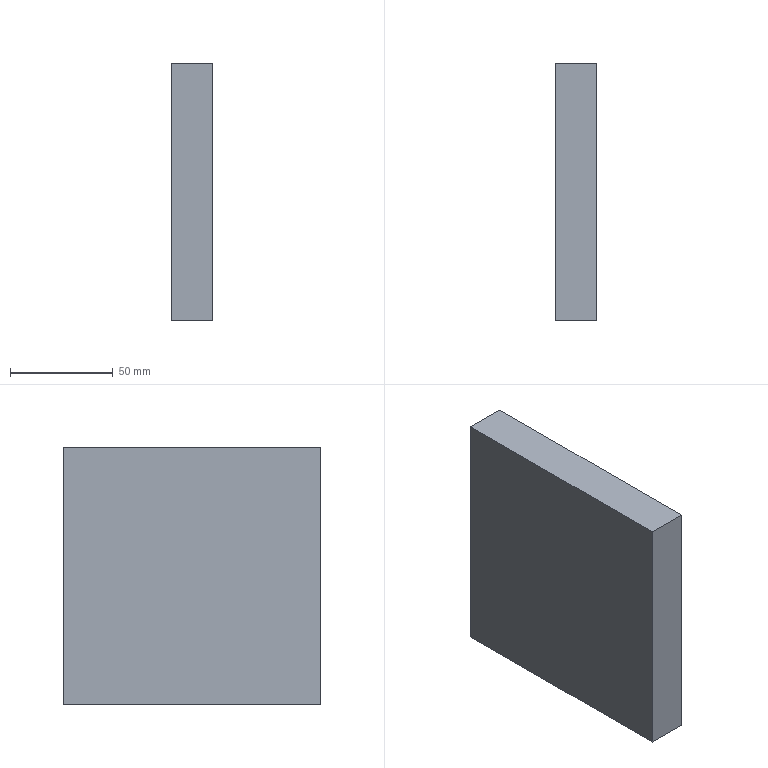Part | NX | features solid 2 | 1 solid | 6 faces | box 20 x 125 x 125 mm | volume 312500 mm3 | plane 6
STEP:
#1=CARTESIAN_POINT('',(-965.,892.5,-65.));
#2=VERTEX_POINT('',#1);
#3=CARTESIAN_POINT('',(-965.,1017.5,-65.));
#4=VERTEX_POINT('',#3);
#5=CARTESIAN_POINT('',(-965.,905.,-65.));
#6=DIRECTION('',(0.,1.,0.));
#7=VECTOR('',#6,1000.);
#8=LINE('',#5,#7);
#9=EDGE_CURVE('',#2,#4,#8,.T.);
#10=ORIENTED_EDGE('',*,*,#9,.T.);
#11=CARTESIAN_POINT('',(-985.,1017.5,-65.));
#12=VERTEX_POINT('',#11);
#13=CARTESIAN_POINT('',(-985.,1017.5,-65.));
#14=DIRECTION('',(1.,0.,0.));
#15=VECTOR('',#14,1000.);
#16=LINE('',#13,#15);
#17=EDGE_CURVE('',#12,#4,#16,.T.);
#18=ORIENTED_EDGE('',*,*,#17,.F.);
#19=CARTESIAN_POINT('',(-985.,892.5,-65.));
#20=VERTEX_POINT('',#19);
#21=CARTESIAN_POINT('',(-985.,905.,-65.));
#22=DIRECTION('',(0.,1.,0.));
#23=VECTOR('',#22,1000.);
#24=LINE('',#21,#23);
#25=EDGE_CURVE('',#20,#12,#24,.T.);
#26=ORIENTED_EDGE('',*,*,#25,.F.);
#27=CARTESIAN_POINT('',(-985.,892.5,-65.));
#28=DIRECTION('',(1.,0.,0.));
#29=VECTOR('',#28,1000.);
#30=LINE('',#27,#29);
#31=EDGE_CURVE('',#20,#2,#30,.T.);
#32=ORIENTED_EDGE('',*,*,#31,.T.);
#33=EDGE_LOOP('',(#10,#18,#26,#32));
#34=FACE_BOUND('',#33,.T.);
#35=CARTESIAN_POINT('',(-985.,905.,-65.));
#36=DIRECTION('',(0.,0.,1.));
#37=DIRECTION('',(0.,-1.,0.));
#38=AXIS2_PLACEMENT_3D('',#35,#36,#37);
#39=PLANE('',#38);
#40=ADVANCED_FACE('',(#34),#39,.T.);
#41=CARTESIAN_POINT('',(-965.,1017.5,-190.));
#42=VERTEX_POINT('',#41);
#43=CARTESIAN_POINT('',(-965.,1017.5,-77.5));
#44=DIRECTION('',(0.,0.,-1.));
#45=VECTOR('',#44,1000.);
#46=LINE('',#43,#45);
#47=EDGE_CURVE('',#4,#42,#46,.T.);
#48=ORIENTED_EDGE('',*,*,#47,.T.);
#49=CARTESIAN_POINT('',(-985.,1017.5,-190.));
#50=VERTEX_POINT('',#49);
#51=CARTESIAN_POINT('',(-985.,1017.5,-190.));
#52=DIRECTION('',(1.,0.,0.));
#53=VECTOR('',#52,1000.);
#54=LINE('',#51,#53);
#55=EDGE_CURVE('',#50,#42,#54,.T.);
#56=ORIENTED_EDGE('',*,*,#55,.F.);
#57=CARTESIAN_POINT('',(-985.,1017.5,-77.5));
#58=DIRECTION('',(0.,0.,-1.));
#59=VECTOR('',#58,1000.);
#60=LINE('',#57,#59);
#61=EDGE_CURVE('',#12,#50,#60,.T.);
#62=ORIENTED_EDGE('',*,*,#61,.F.);
#63=ORIENTED_EDGE('',*,*,#17,.T.);
#64=EDGE_LOOP('',(#48,#56,#62,#63));
#65=FACE_BOUND('',#64,.T.);
#66=CARTESIAN_POINT('',(-985.,1017.5,-77.5));
#67=DIRECTION('',(0.,1.,0.));
#68=DIRECTION('',(0.,0.,1.));
#69=AXIS2_PLACEMENT_3D('',#66,#67,#68);
#70=PLANE('',#69);
#71=ADVANCED_FACE('',(#65),#70,.T.);
#72=CARTESIAN_POINT('',(-965.,892.5,-190.));
#73=VERTEX_POINT('',#72);
#74=CARTESIAN_POINT('',(-965.,1005.,-190.));
#75=DIRECTION('',(0.,-1.,0.));
#76=VECTOR('',#75,1000.);
#77=LINE('',#74,#76);
#78=EDGE_CURVE('',#42,#73,#77,.T.);
#79=ORIENTED_EDGE('',*,*,#78,.T.);
#80=CARTESIAN_POINT('',(-985.,892.5,-190.));
#81=VERTEX_POINT('',#80);
#82=CARTESIAN_POINT('',(-985.,892.5,-190.));
#83=DIRECTION('',(1.,0.,0.));
#84=VECTOR('',#83,1000.);
#85=LINE('',#82,#84);
#86=EDGE_CURVE('',#81,#73,#85,.T.);
#87=ORIENTED_EDGE('',*,*,#86,.F.);
#88=CARTESIAN_POINT('',(-985.,1005.,-190.));
#89=DIRECTION('',(0.,-1.,0.));
#90=VECTOR('',#89,1000.);
#91=LINE('',#88,#90);
#92=EDGE_CURVE('',#50,#81,#91,.T.);
#93=ORIENTED_EDGE('',*,*,#92,.F.);
#94=ORIENTED_EDGE('',*,*,#55,.T.);
#95=EDGE_LOOP('',(#79,#87,#93,#94));
#96=FACE_BOUND('',#95,.T.);
#97=CARTESIAN_POINT('',(-985.,1005.,-190.));
#98=DIRECTION('',(0.,0.,-1.));
#99=DIRECTION('',(1.,0.,0.));
#100=AXIS2_PLACEMENT_3D('',#97,#98,#99);
#101=PLANE('',#100);
#102=ADVANCED_FACE('',(#96),#101,.T.);
#103=CARTESIAN_POINT('',(-965.,892.5,-177.5));
#104=DIRECTION('',(0.,0.,1.));
#105=VECTOR('',#104,1000.);
#106=LINE('',#103,#105);
#107=EDGE_CURVE('',#73,#2,#106,.T.);
#108=ORIENTED_EDGE('',*,*,#107,.T.);
#109=ORIENTED_EDGE('',*,*,#31,.F.);
#110=CARTESIAN_POINT('',(-985.,892.5,-177.5));
#111=DIRECTION('',(0.,0.,1.));
#112=VECTOR('',#111,1000.);
#113=LINE('',#110,#112);
#114=EDGE_CURVE('',#81,#20,#113,.T.);
#115=ORIENTED_EDGE('',*,*,#114,.F.);
#116=ORIENTED_EDGE('',*,*,#86,.T.);
#117=EDGE_LOOP('',(#108,#109,#115,#116));
#118=FACE_BOUND('',#117,.T.);
#119=CARTESIAN_POINT('',(-985.,892.5,-177.5));
#120=DIRECTION('',(0.,-1.,0.));
#121=DIRECTION('',(-1.,0.,0.));
#122=AXIS2_PLACEMENT_3D('',#119,#120,#121);
#123=PLANE('',#122);
#124=ADVANCED_FACE('',(#118),#123,.T.);
#125=ORIENTED_EDGE('',*,*,#25,.T.);
#126=ORIENTED_EDGE('',*,*,#61,.T.);
#127=ORIENTED_EDGE('',*,*,#92,.T.);
#128=ORIENTED_EDGE('',*,*,#114,.T.);
#129=EDGE_LOOP('',(#125,#126,#127,#128));
#130=FACE_BOUND('',#129,.T.);
#131=CARTESIAN_POINT('',(-985.,905.,-77.5));
#132=DIRECTION('',(-1.,0.,0.));
#133=DIRECTION('',(0.,1.,0.));
#134=AXIS2_PLACEMENT_3D('',#131,#132,#133);
#135=PLANE('',#134);
#136=ADVANCED_FACE('',(#130),#135,.T.);
#137=ORIENTED_EDGE('',*,*,#9,.F.);
#138=ORIENTED_EDGE('',*,*,#107,.F.);
#139=ORIENTED_EDGE('',*,*,#78,.F.);
#140=ORIENTED_EDGE('',*,*,#47,.F.);
#141=EDGE_LOOP('',(#137,#138,#139,#140));
#142=FACE_BOUND('',#141,.T.);
#143=CARTESIAN_POINT('',(-965.,905.,-77.5));
#144=DIRECTION('',(-1.,0.,0.));
#145=DIRECTION('',(0.,1.,0.));
#146=AXIS2_PLACEMENT_3D('',#143,#144,#145);
#147=PLANE('',#146);
#148=ADVANCED_FACE('',(#142),#147,.F.);
#149=CLOSED_SHELL('',(#40,#71,#102,#124,#136,#148));
#150=MANIFOLD_SOLID_BREP('',#149);
#151=(LENGTH_UNIT()NAMED_UNIT(*)SI_UNIT(.MILLI.,.METRE.));
#152=UNCERTAINTY_MEASURE_WITH_UNIT(LENGTH_MEASURE(0.00001),#151,'','');
#153=(NAMED_UNIT(*)PLANE_ANGLE_UNIT()SI_UNIT($,.RADIAN.));
#154=(NAMED_UNIT(*)SI_UNIT($,.STERADIAN.)SOLID_ANGLE_UNIT());
#155=(GEOMETRIC_REPRESENTATION_CONTEXT(3)GLOBAL_UNCERTAINTY_ASSIGNED_CONTEXT((#152))GLOBAL_UNIT_ASSIGNED_CONTEXT((#151,#153,#154))REPRESENTATION_CONTEXT('',''));
#156=ADVANCED_BREP_SHAPE_REPRESENTATION('',(#150),#155);